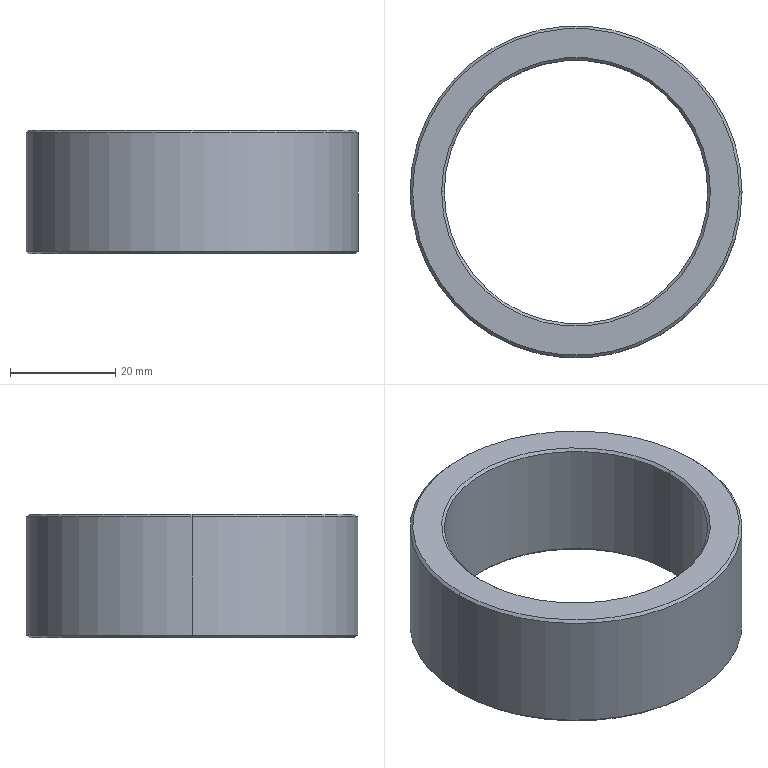Part | SolidWorks | features Chamfer 1, Extrusion 1 | 1 solid | 14 faces | box 63 x 63 x 23.5 mm | volume 27024 mm3 | cone 8 | cylinder 4 | plane 2 | commonest cylinder face diameters 50 x2 63 x2
STEP:
#1=CARTESIAN_POINT('',(31.,0.,23.5));
#2=VERTEX_POINT('',#1);
#3=CARTESIAN_POINT('',(-31.,0.,23.5));
#4=VERTEX_POINT('',#3);
#5=CARTESIAN_POINT('',(0.,0.,23.5));
#6=DIRECTION('',(0.,0.,1.));
#7=DIRECTION('',(1.,0.,0.));
#8=AXIS2_PLACEMENT_3D('',#5,#6,#7);
#9=CIRCLE('',#8,31.);
#10=EDGE_CURVE('',#2,#4,#9,.T.);
#11=ORIENTED_EDGE('',*,*,#10,.F.);
#12=CARTESIAN_POINT('',(31.5,0.,23.));
#13=VERTEX_POINT('',#12);
#14=CARTESIAN_POINT('',(31.,0.,23.5));
#15=DIRECTION('',(0.7071,0.,-0.7071));
#16=VECTOR('',#15,1000.);
#17=LINE('',#14,#16);
#18=EDGE_CURVE('',#2,#13,#17,.T.);
#19=ORIENTED_EDGE('',*,*,#18,.T.);
#20=CARTESIAN_POINT('',(-31.5,0.,23.));
#21=VERTEX_POINT('',#20);
#22=CARTESIAN_POINT('',(0.,0.,23.));
#23=DIRECTION('',(0.,0.,-1.));
#24=DIRECTION('',(1.,0.,0.));
#25=AXIS2_PLACEMENT_3D('',#22,#23,#24);
#26=CIRCLE('',#25,31.5);
#27=EDGE_CURVE('',#21,#13,#26,.T.);
#28=ORIENTED_EDGE('',*,*,#27,.F.);
#29=CARTESIAN_POINT('',(-31.,0.,23.5));
#30=DIRECTION('',(-0.7071,0.,-0.7071));
#31=VECTOR('',#30,1000.);
#32=LINE('',#29,#31);
#33=EDGE_CURVE('',#4,#21,#32,.T.);
#34=ORIENTED_EDGE('',*,*,#33,.F.);
#35=EDGE_LOOP('',(#11,#19,#28,#34));
#36=FACE_OUTER_BOUND('',#35,.T.);
#37=CARTESIAN_POINT('',(0.,0.,23.5));
#38=DIRECTION('',(0.,0.,-1.));
#39=DIRECTION('',(-1.,0.,0.));
#40=AXIS2_PLACEMENT_3D('',#37,#38,#39);
#41=CONICAL_SURFACE('',#40,31.,0.7854);
#42=ADVANCED_FACE('',(#36),#41,.T.);
#43=CARTESIAN_POINT('',(-25.,0.,23.));
#44=VERTEX_POINT('',#43);
#45=CARTESIAN_POINT('',(25.,0.,23.));
#46=VERTEX_POINT('',#45);
#47=CARTESIAN_POINT('',(0.,0.,23.));
#48=DIRECTION('',(0.,0.,1.));
#49=DIRECTION('',(1.,0.,0.));
#50=AXIS2_PLACEMENT_3D('',#47,#48,#49);
#51=CIRCLE('',#50,25.);
#52=EDGE_CURVE('',#44,#46,#51,.T.);
#53=ORIENTED_EDGE('',*,*,#52,.F.);
#54=CARTESIAN_POINT('',(-25.5,0.,23.5));
#55=VERTEX_POINT('',#54);
#56=CARTESIAN_POINT('',(-25.,0.,23.));
#57=DIRECTION('',(-0.7071,0.,0.7071));
#58=VECTOR('',#57,1000.);
#59=LINE('',#56,#58);
#60=EDGE_CURVE('',#44,#55,#59,.T.);
#61=ORIENTED_EDGE('',*,*,#60,.T.);
#62=CARTESIAN_POINT('',(25.5,0.,23.5));
#63=VERTEX_POINT('',#62);
#64=CARTESIAN_POINT('',(0.,0.,23.5));
#65=DIRECTION('',(0.,0.,-1.));
#66=DIRECTION('',(1.,0.,0.));
#67=AXIS2_PLACEMENT_3D('',#64,#65,#66);
#68=CIRCLE('',#67,25.5);
#69=EDGE_CURVE('',#63,#55,#68,.T.);
#70=ORIENTED_EDGE('',*,*,#69,.F.);
#71=CARTESIAN_POINT('',(25.,0.,23.));
#72=DIRECTION('',(0.7071,0.,0.7071));
#73=VECTOR('',#72,1000.);
#74=LINE('',#71,#73);
#75=EDGE_CURVE('',#46,#63,#74,.T.);
#76=ORIENTED_EDGE('',*,*,#75,.F.);
#77=EDGE_LOOP('',(#53,#61,#70,#76));
#78=FACE_OUTER_BOUND('',#77,.T.);
#79=CARTESIAN_POINT('',(0.,0.,23.));
#80=DIRECTION('',(0.,0.,1.));
#81=DIRECTION('',(1.,0.,0.));
#82=AXIS2_PLACEMENT_3D('',#79,#80,#81);
#83=CONICAL_SURFACE('',#82,25.,0.7854);
#84=ADVANCED_FACE('',(#78),#83,.F.);
#85=CARTESIAN_POINT('',(-31.,0.,0.));
#86=VERTEX_POINT('',#85);
#87=CARTESIAN_POINT('',(31.,0.,0.));
#88=VERTEX_POINT('',#87);
#89=CARTESIAN_POINT('',(0.,0.,0.));
#90=DIRECTION('',(0.,0.,-1.));
#91=DIRECTION('',(1.,0.,0.));
#92=AXIS2_PLACEMENT_3D('',#89,#90,#91);
#93=CIRCLE('',#92,31.);
#94=EDGE_CURVE('',#86,#88,#93,.T.);
#95=ORIENTED_EDGE('',*,*,#94,.F.);
#96=CARTESIAN_POINT('',(-31.5,0.,0.5));
#97=VERTEX_POINT('',#96);
#98=CARTESIAN_POINT('',(-31.5,0.,0.5));
#99=DIRECTION('',(-0.7071,0.,0.7071));
#100=VECTOR('',#99,1000.);
#101=LINE('',#98,#100);
#102=EDGE_CURVE('',#86,#97,#101,.T.);
#103=ORIENTED_EDGE('',*,*,#102,.T.);
#104=CARTESIAN_POINT('',(31.5,0.,0.5));
#105=VERTEX_POINT('',#104);
#106=CARTESIAN_POINT('',(0.,0.,0.5));
#107=DIRECTION('',(0.,0.,1.));
#108=DIRECTION('',(1.,0.,0.));
#109=AXIS2_PLACEMENT_3D('',#106,#107,#108);
#110=CIRCLE('',#109,31.5);
#111=EDGE_CURVE('',#105,#97,#110,.T.);
#112=ORIENTED_EDGE('',*,*,#111,.F.);
#113=CARTESIAN_POINT('',(31.5,0.,0.5));
#114=DIRECTION('',(0.7071,0.,0.7071));
#115=VECTOR('',#114,1000.);
#116=LINE('',#113,#115);
#117=EDGE_CURVE('',#88,#105,#116,.T.);
#118=ORIENTED_EDGE('',*,*,#117,.F.);
#119=EDGE_LOOP('',(#95,#103,#112,#118));
#120=FACE_OUTER_BOUND('',#119,.T.);
#121=CARTESIAN_POINT('',(0.,0.,0.5));
#122=DIRECTION('',(0.,0.,1.));
#123=DIRECTION('',(1.,0.,0.));
#124=AXIS2_PLACEMENT_3D('',#121,#122,#123);
#125=CONICAL_SURFACE('',#124,31.5,0.7854);
#126=ADVANCED_FACE('',(#120),#125,.T.);
#127=CARTESIAN_POINT('',(25.,0.,0.5));
#128=VERTEX_POINT('',#127);
#129=CARTESIAN_POINT('',(-25.,0.,0.5));
#130=VERTEX_POINT('',#129);
#131=CARTESIAN_POINT('',(0.,0.,0.5));
#132=DIRECTION('',(0.,0.,-1.));
#133=DIRECTION('',(1.,0.,0.));
#134=AXIS2_PLACEMENT_3D('',#131,#132,#133);
#135=CIRCLE('',#134,25.);
#136=EDGE_CURVE('',#128,#130,#135,.T.);
#137=ORIENTED_EDGE('',*,*,#136,.F.);
#138=CARTESIAN_POINT('',(25.5,0.,0.));
#139=VERTEX_POINT('',#138);
#140=CARTESIAN_POINT('',(25.5,0.,0.));
#141=DIRECTION('',(0.7071,0.,-0.7071));
#142=VECTOR('',#141,1000.);
#143=LINE('',#140,#142);
#144=EDGE_CURVE('',#128,#139,#143,.T.);
#145=ORIENTED_EDGE('',*,*,#144,.T.);
#146=CARTESIAN_POINT('',(-25.5,0.,0.));
#147=VERTEX_POINT('',#146);
#148=CARTESIAN_POINT('',(0.,0.,0.));
#149=DIRECTION('',(0.,0.,1.));
#150=DIRECTION('',(1.,0.,0.));
#151=AXIS2_PLACEMENT_3D('',#148,#149,#150);
#152=CIRCLE('',#151,25.5);
#153=EDGE_CURVE('',#147,#139,#152,.T.);
#154=ORIENTED_EDGE('',*,*,#153,.F.);
#155=CARTESIAN_POINT('',(-25.5,0.,0.));
#156=DIRECTION('',(-0.7071,0.,-0.7071));
#157=VECTOR('',#156,1000.);
#158=LINE('',#155,#157);
#159=EDGE_CURVE('',#130,#147,#158,.T.);
#160=ORIENTED_EDGE('',*,*,#159,.F.);
#161=EDGE_LOOP('',(#137,#145,#154,#160));
#162=FACE_OUTER_BOUND('',#161,.T.);
#163=CARTESIAN_POINT('',(0.,0.,0.));
#164=DIRECTION('',(0.,0.,-1.));
#165=DIRECTION('',(-1.,0.,0.));
#166=AXIS2_PLACEMENT_3D('',#163,#164,#165);
#167=CONICAL_SURFACE('',#166,25.5,0.7854);
#168=ADVANCED_FACE('',(#162),#167,.F.);
#169=ORIENTED_EDGE('',*,*,#52,.T.);
#170=CARTESIAN_POINT('',(25.,0.,23.5));
#171=DIRECTION('',(0.,0.,-1.));
#172=VECTOR('',#171,1000.);
#173=LINE('',#170,#172);
#174=EDGE_CURVE('',#46,#128,#173,.T.);
#175=ORIENTED_EDGE('',*,*,#174,.T.);
#176=ORIENTED_EDGE('',*,*,#136,.T.);
#177=CARTESIAN_POINT('',(-25.,0.,23.5));
#178=DIRECTION('',(0.,0.,-1.));
#179=VECTOR('',#178,1000.);
#180=LINE('',#177,#179);
#181=EDGE_CURVE('',#44,#130,#180,.T.);
#182=ORIENTED_EDGE('',*,*,#181,.F.);
#183=EDGE_LOOP('',(#169,#175,#176,#182));
#184=FACE_OUTER_BOUND('',#183,.T.);
#185=CARTESIAN_POINT('',(0.,0.,23.5));
#186=DIRECTION('',(0.,0.,-1.));
#187=DIRECTION('',(-1.,0.,0.));
#188=AXIS2_PLACEMENT_3D('',#185,#186,#187);
#189=CYLINDRICAL_SURFACE('',#188,25.);
#190=ADVANCED_FACE('',(#184),#189,.F.);
#191=ORIENTED_EDGE('',*,*,#27,.T.);
#192=CARTESIAN_POINT('',(31.5,0.,23.5));
#193=DIRECTION('',(0.,0.,-1.));
#194=VECTOR('',#193,1000.);
#195=LINE('',#192,#194);
#196=EDGE_CURVE('',#13,#105,#195,.T.);
#197=ORIENTED_EDGE('',*,*,#196,.T.);
#198=ORIENTED_EDGE('',*,*,#111,.T.);
#199=CARTESIAN_POINT('',(-31.5,0.,23.5));
#200=DIRECTION('',(0.,0.,-1.));
#201=VECTOR('',#200,1000.);
#202=LINE('',#199,#201);
#203=EDGE_CURVE('',#21,#97,#202,.T.);
#204=ORIENTED_EDGE('',*,*,#203,.F.);
#205=EDGE_LOOP('',(#191,#197,#198,#204));
#206=FACE_OUTER_BOUND('',#205,.T.);
#207=CARTESIAN_POINT('',(0.,0.,23.5));
#208=DIRECTION('',(0.,0.,-1.));
#209=DIRECTION('',(-1.,0.,0.));
#210=AXIS2_PLACEMENT_3D('',#207,#208,#209);
#211=CYLINDRICAL_SURFACE('',#210,31.5);
#212=ADVANCED_FACE('',(#206),#211,.T.);
#213=ORIENTED_EDGE('',*,*,#69,.T.);
#214=CARTESIAN_POINT('',(0.,0.,23.5));
#215=DIRECTION('',(0.,0.,-1.));
#216=DIRECTION('',(1.,0.,0.));
#217=AXIS2_PLACEMENT_3D('',#214,#215,#216);
#218=CIRCLE('',#217,25.5);
#219=EDGE_CURVE('',#55,#63,#218,.T.);
#220=ORIENTED_EDGE('',*,*,#219,.T.);
#221=EDGE_LOOP('',(#213,#220));
#222=FACE_BOUND('',#221,.T.);
#223=CARTESIAN_POINT('',(0.,0.,23.5));
#224=DIRECTION('',(0.,0.,1.));
#225=DIRECTION('',(1.,0.,0.));
#226=AXIS2_PLACEMENT_3D('',#223,#224,#225);
#227=CIRCLE('',#226,31.);
#228=EDGE_CURVE('',#4,#2,#227,.T.);
#229=ORIENTED_EDGE('',*,*,#228,.T.);
#230=ORIENTED_EDGE('',*,*,#10,.T.);
#231=EDGE_LOOP('',(#229,#230));
#232=FACE_OUTER_BOUND('',#231,.T.);
#233=CARTESIAN_POINT('',(0.,0.,23.5));
#234=DIRECTION('',(0.,0.,1.));
#235=DIRECTION('',(1.,0.,0.));
#236=AXIS2_PLACEMENT_3D('',#233,#234,#235);
#237=PLANE('',#236);
#238=ADVANCED_FACE('',(#222,#232),#237,.T.);
#239=ORIENTED_EDGE('',*,*,#153,.T.);
#240=CARTESIAN_POINT('',(0.,0.,0.));
#241=DIRECTION('',(0.,0.,1.));
#242=DIRECTION('',(1.,0.,0.));
#243=AXIS2_PLACEMENT_3D('',#240,#241,#242);
#244=CIRCLE('',#243,25.5);
#245=EDGE_CURVE('',#139,#147,#244,.T.);
#246=ORIENTED_EDGE('',*,*,#245,.T.);
#247=EDGE_LOOP('',(#239,#246));
#248=FACE_BOUND('',#247,.T.);
#249=CARTESIAN_POINT('',(0.,0.,0.));
#250=DIRECTION('',(0.,0.,-1.));
#251=DIRECTION('',(1.,0.,0.));
#252=AXIS2_PLACEMENT_3D('',#249,#250,#251);
#253=CIRCLE('',#252,31.);
#254=EDGE_CURVE('',#88,#86,#253,.T.);
#255=ORIENTED_EDGE('',*,*,#254,.T.);
#256=ORIENTED_EDGE('',*,*,#94,.T.);
#257=EDGE_LOOP('',(#255,#256));
#258=FACE_OUTER_BOUND('',#257,.T.);
#259=CARTESIAN_POINT('',(0.,0.,0.));
#260=DIRECTION('',(0.,0.,1.));
#261=DIRECTION('',(1.,0.,0.));
#262=AXIS2_PLACEMENT_3D('',#259,#260,#261);
#263=PLANE('',#262);
#264=ADVANCED_FACE('',(#248,#258),#263,.F.);
#265=ORIENTED_EDGE('',*,*,#196,.F.);
#266=CARTESIAN_POINT('',(0.,0.,23.));
#267=DIRECTION('',(0.,0.,-1.));
#268=DIRECTION('',(1.,0.,0.));
#269=AXIS2_PLACEMENT_3D('',#266,#267,#268);
#270=CIRCLE('',#269,31.5);
#271=EDGE_CURVE('',#13,#21,#270,.T.);
#272=ORIENTED_EDGE('',*,*,#271,.T.);
#273=ORIENTED_EDGE('',*,*,#203,.T.);
#274=CARTESIAN_POINT('',(0.,0.,0.5));
#275=DIRECTION('',(0.,0.,1.));
#276=DIRECTION('',(1.,0.,0.));
#277=AXIS2_PLACEMENT_3D('',#274,#275,#276);
#278=CIRCLE('',#277,31.5);
#279=EDGE_CURVE('',#97,#105,#278,.T.);
#280=ORIENTED_EDGE('',*,*,#279,.T.);
#281=EDGE_LOOP('',(#265,#272,#273,#280));
#282=FACE_OUTER_BOUND('',#281,.T.);
#283=CARTESIAN_POINT('',(0.,0.,23.5));
#284=DIRECTION('',(0.,0.,-1.));
#285=DIRECTION('',(-1.,0.,0.));
#286=AXIS2_PLACEMENT_3D('',#283,#284,#285);
#287=CYLINDRICAL_SURFACE('',#286,31.5);
#288=ADVANCED_FACE('',(#282),#287,.T.);
#289=ORIENTED_EDGE('',*,*,#174,.F.);
#290=CARTESIAN_POINT('',(0.,0.,23.));
#291=DIRECTION('',(0.,0.,1.));
#292=DIRECTION('',(1.,0.,0.));
#293=AXIS2_PLACEMENT_3D('',#290,#291,#292);
#294=CIRCLE('',#293,25.);
#295=EDGE_CURVE('',#46,#44,#294,.T.);
#296=ORIENTED_EDGE('',*,*,#295,.T.);
#297=ORIENTED_EDGE('',*,*,#181,.T.);
#298=CARTESIAN_POINT('',(0.,0.,0.5));
#299=DIRECTION('',(0.,0.,-1.));
#300=DIRECTION('',(1.,0.,0.));
#301=AXIS2_PLACEMENT_3D('',#298,#299,#300);
#302=CIRCLE('',#301,25.);
#303=EDGE_CURVE('',#130,#128,#302,.T.);
#304=ORIENTED_EDGE('',*,*,#303,.T.);
#305=EDGE_LOOP('',(#289,#296,#297,#304));
#306=FACE_OUTER_BOUND('',#305,.T.);
#307=CARTESIAN_POINT('',(0.,0.,23.5));
#308=DIRECTION('',(0.,0.,-1.));
#309=DIRECTION('',(-1.,0.,0.));
#310=AXIS2_PLACEMENT_3D('',#307,#308,#309);
#311=CYLINDRICAL_SURFACE('',#310,25.);
#312=ADVANCED_FACE('',(#306),#311,.F.);
#313=ORIENTED_EDGE('',*,*,#144,.F.);
#314=ORIENTED_EDGE('',*,*,#303,.F.);
#315=ORIENTED_EDGE('',*,*,#159,.T.);
#316=ORIENTED_EDGE('',*,*,#245,.F.);
#317=EDGE_LOOP('',(#313,#314,#315,#316));
#318=FACE_OUTER_BOUND('',#317,.T.);
#319=CARTESIAN_POINT('',(0.,0.,0.));
#320=DIRECTION('',(0.,0.,-1.));
#321=DIRECTION('',(-1.,0.,0.));
#322=AXIS2_PLACEMENT_3D('',#319,#320,#321);
#323=CONICAL_SURFACE('',#322,25.5,0.7854);
#324=ADVANCED_FACE('',(#318),#323,.F.);
#325=ORIENTED_EDGE('',*,*,#102,.F.);
#326=ORIENTED_EDGE('',*,*,#254,.F.);
#327=ORIENTED_EDGE('',*,*,#117,.T.);
#328=ORIENTED_EDGE('',*,*,#279,.F.);
#329=EDGE_LOOP('',(#325,#326,#327,#328));
#330=FACE_OUTER_BOUND('',#329,.T.);
#331=CARTESIAN_POINT('',(0.,0.,0.5));
#332=DIRECTION('',(0.,0.,1.));
#333=DIRECTION('',(1.,0.,0.));
#334=AXIS2_PLACEMENT_3D('',#331,#332,#333);
#335=CONICAL_SURFACE('',#334,31.5,0.7854);
#336=ADVANCED_FACE('',(#330),#335,.T.);
#337=ORIENTED_EDGE('',*,*,#60,.F.);
#338=ORIENTED_EDGE('',*,*,#295,.F.);
#339=ORIENTED_EDGE('',*,*,#75,.T.);
#340=ORIENTED_EDGE('',*,*,#219,.F.);
#341=EDGE_LOOP('',(#337,#338,#339,#340));
#342=FACE_OUTER_BOUND('',#341,.T.);
#343=CARTESIAN_POINT('',(0.,0.,23.));
#344=DIRECTION('',(0.,0.,1.));
#345=DIRECTION('',(1.,0.,0.));
#346=AXIS2_PLACEMENT_3D('',#343,#344,#345);
#347=CONICAL_SURFACE('',#346,25.,0.7854);
#348=ADVANCED_FACE('',(#342),#347,.F.);
#349=ORIENTED_EDGE('',*,*,#18,.F.);
#350=ORIENTED_EDGE('',*,*,#228,.F.);
#351=ORIENTED_EDGE('',*,*,#33,.T.);
#352=ORIENTED_EDGE('',*,*,#271,.F.);
#353=EDGE_LOOP('',(#349,#350,#351,#352));
#354=FACE_OUTER_BOUND('',#353,.T.);
#355=CARTESIAN_POINT('',(0.,0.,23.5));
#356=DIRECTION('',(0.,0.,-1.));
#357=DIRECTION('',(-1.,0.,0.));
#358=AXIS2_PLACEMENT_3D('',#355,#356,#357);
#359=CONICAL_SURFACE('',#358,31.,0.7854);
#360=ADVANCED_FACE('',(#354),#359,.T.);
#361=CLOSED_SHELL('',(#42,#84,#126,#168,#190,#212,#238,#264,#288,#312,#324,#336,#348,#360));
#362=MANIFOLD_SOLID_BREP('',#361);
#363=CARTESIAN_POINT('',(0.,0.,0.));
#364=DIRECTION('',(0.,0.,1.));
#365=DIRECTION('',(1.,0.,0.));
#366=AXIS2_PLACEMENT_3D('',#363,#364,#365);
#367=(LENGTH_UNIT()NAMED_UNIT(*)SI_UNIT(.MILLI.,.METRE.));
#368=UNCERTAINTY_MEASURE_WITH_UNIT(LENGTH_MEASURE(0.00001),#367,'','');
#369=(NAMED_UNIT(*)PLANE_ANGLE_UNIT()SI_UNIT($,.RADIAN.));
#370=(NAMED_UNIT(*)SI_UNIT($,.STERADIAN.)SOLID_ANGLE_UNIT());
#371=(GEOMETRIC_REPRESENTATION_CONTEXT(3)GLOBAL_UNCERTAINTY_ASSIGNED_CONTEXT((#368))GLOBAL_UNIT_ASSIGNED_CONTEXT((#367,#369,#370))REPRESENTATION_CONTEXT('',''));
#372=ADVANCED_BREP_SHAPE_REPRESENTATION('',(#362,#366),#371);